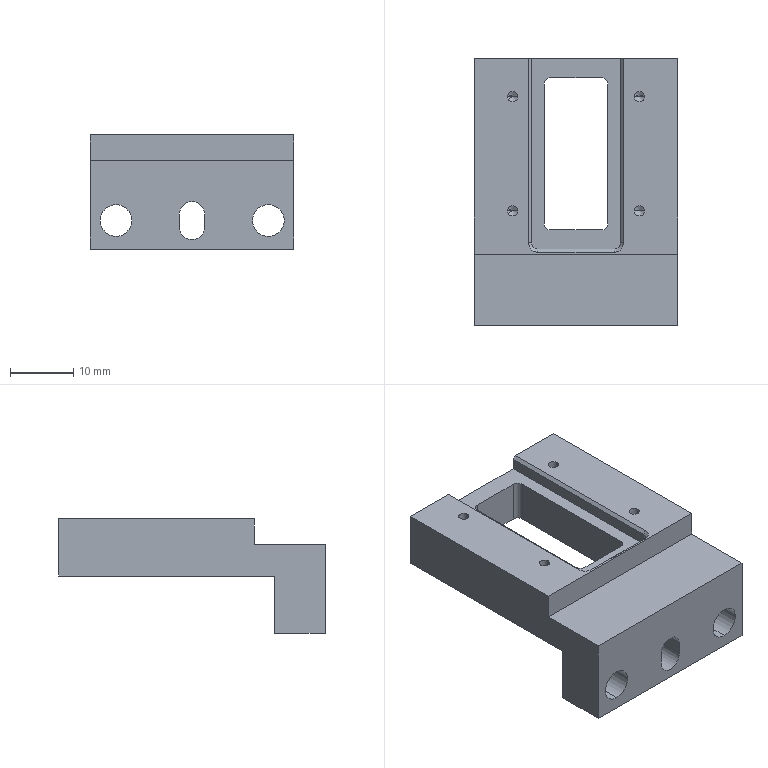NC program | NX | posted with a generic post | part box 32 x 42 x 18 mm
Whole program:
N10 G17 G21 G94 G90
(FLOOR_WALL , TOOL : D10JING)
N12 T11 M6
N14 G54
N16 G17 G0 G90 X-31. Y17.997 B0. C0. S9500 M3
N18 G43 Z30. H11
N20 Z3.
N22 G94 G1 Z0. F1250.
N24 X-28.
N26 X28.
N28 Y13.426
N30 X-28.
N32 Y8.855
N34 X28.
N36 Y4.284
N38 X-28.
N40 Y-0.287
N42 X28.
N44 Y-4.858
N46 X-28.
N48 Y-9.429
N50 X28.
N52 Y-14.
N54 X-28.
N56 X-31.
N58 Z3.
N60 G0 Z30.
N62 M5
(DRILLING , TOOL : D6A45)
N64 T07 M6
N66 G54
N68 G17 G0 G90 X-2.991 Y-10. B0. C0. S5000 M3
N70 G43 Z30. H7
N72 G94 G81 G98 Z-1. F250. R3.
N74 X15.009
N76 Y10.
N78 X-2.991
N80 G80
N82 G0 X-2.991 Y10. Z30.
N84 M5
(DRILLING_COPY , TOOL : 1.6ZT)
N86 T14 M6
N88 G54
N90 G17 G0 G90 X-2.991 Y-10. B0. C0. S2009 M3
N92 G43 Z30. H14
N94 G94 G83 G98 Z-5.681 F100. Q2. R3.
N96 X15.009
N98 Y10.
N100 X-2.991
N102 G80
N104 G0 X-2.991 Y10. Z30.
N106 M5
(ZLEVEL_PROFILE , TOOL : D10)
N108 T10 M6
N110 G54
N112 G17 G0 G90 X-26.1 Y-14.091 B0. C0. S9500 M3
N114 G43 Z30. H10
N116 Z1.5
N118 G94 G1 Y16.32 Z-0.094 F1000.
N120 X-25.983 Y17.131 Z-0.137
N122 X-25.738 Y17.914 Z-0.18
N124 X-25.371 Y18.647 Z-0.223
N126 X-24.892 Y19.312 Z-0.266
N128 X-24.312 Y19.892 Z-0.309
N130 X-23.647 Y20.371 Z-0.352
N132 X-22.914 Y20.738 Z-0.395
N134 X-22.131 Y20.983 Z-0.438
N136 X-21.32 Y21.1 Z-0.48
N138 X-21. Z-0.497
N140 X21. F3000.
N142 G2 X26.1 Y16. R5.1
N144 G1 Y-16.
N146 G2 X21. Y-21.1 R5.1
N148 G1 X-21.
N150 G2 X-26.1 Y-16. R5.1
N152 G1 Y16.
N154 G2 X-21. Y21.1 R5.1
N156 G1 X7.486 Z-0.994
N158 X21.
N160 G2 X26.1 Y16. R5.1
N162 G1 Y-16.
N164 G2 X21. Y-21.1 R5.1
N166 G1 X-21.
N168 G2 X-26.1 Y-16. R5.1
N170 G1 Y16.
N172 G2 X-21. Y21.1 R5.1
N174 G1 X7.486 Z-1.492
N176 X21.
N178 G2 X26.1 Y16. R5.1
N180 G1 Y-16.
N182 G2 X21. Y-21.1 R5.1
N184 G1 X-21.
N186 G2 X-26.1 Y-16. R5.1
N188 G1 Y16.
N190 G2 X-21. Y21.1 R5.1
N192 G1 X7.486 Z-1.989
N194 X21.
N196 G2 X26.1 Y16. R5.1
N198 G1 Y-16.
N200 G2 X21. Y-21.1 R5.1
N202 G1 X-21.
N204 G2 X-26.1 Y-16. R5.1
N206 G1 Y16.
N208 G2 X-21. Y21.1 R5.1
N210 G1 X7.486 Z-2.486
N212 X21.
N214 G2 X26.1 Y16. R5.1
N216 G1 Y-16.
N218 G2 X21. Y-21.1 R5.1
N220 G1 X-21.
N222 G2 X-26.1 Y-16. R5.1
N224 G1 Y16.
N226 G2 X-21. Y21.1 R5.1
N228 G1 X7.486 Z-2.983
N230 X21.
N232 G2 X26.1 Y16. R5.1
N234 G1 Y-16.
N236 G2 X21. Y-21.1 R5.1
N238 G1 X-21.
N240 G2 X-26.1 Y-16. R5.1
N242 G1 Y16.
N244 G2 X-21. Y21.1 R5.1
N246 G1 X7.486 Z-3.481
N248 X21.
N250 G2 X26.1 Y16. R5.1
N252 G1 Y-16.
N254 G2 X21. Y-21.1 R5.1
N256 G1 X-21.
N258 G2 X-26.1 Y-16. R5.1
N260 G1 Y16.
N262 G2 X-21. Y21.1 R5.1
N264 G1 X7.486 Z-3.978
N266 X21.
N268 G2 X26.1 Y16. R5.1
N270 G1 Y-16.
N272 G2 X21. Y-21.1 R5.1
N274 G1 X-21.
N276 G2 X-26.1 Y-16. R5.1
N278 G1 Y16.
N280 G2 X-21. Y21.1 R5.1
N282 G1 X7.486 Z-4.475
N284 X21.
N286 G2 X26.1 Y16. R5.1
N288 G1 Y-16.
N290 G2 X21. Y-21.1 R5.1
N292 G1 X-21.
N294 G2 X-26.1 Y-16. R5.1
N296 G1 Y16.
N298 G2 X-21. Y21.1 R5.1
N300 G1 X7.486 Z-4.972
N302 X21.
N304 G2 X26.1 Y16. R5.1
N306 G1 Y-16.
N308 G2 X21. Y-21.1 R5.1
N310 G1 X-21.
N312 G2 X-26.1 Y-16. R5.1
N314 G1 Y16.
N316 G2 X-21. Y21.1 R5.1
N318 G1 X7.486 Z-5.469
N320 X21.
N322 G2 X26.1 Y16. R5.1
N324 G1 Y-16.
N326 G2 X21. Y-21.1 R5.1
N328 G1 X-21.
N330 G2 X-26.1 Y-16. R5.1
N332 G1 Y16.
N334 G2 X-21. Y21.1 R5.1
N336 G1 X7.486 Z-5.967
N338 X21.
N340 G2 X26.1 Y16. R5.1
N342 G1 Y-16.
N344 G2 X21. Y-21.1 R5.1
N346 G1 X-21.
N348 G2 X-26.1 Y-16. R5.1
N350 G1 Y16.
N352 G2 X-21. Y21.1 R5.1
N354 G1 X7.486 Z-6.464
N356 X21.
N358 G2 X26.1 Y16. R5.1
N360 G1 Y-16.
N362 G2 X21. Y-21.1 R5.1
N364 G1 X-21.
N366 G2 X-26.1 Y-16. R5.1
N368 G1 Y16.
N370 G2 X-21. Y21.1 R5.1
N372 G1 X7.486 Z-6.961
N374 X21.
N376 G2 X26.1 Y16. R5.1
N378 G1 Y-16.
N380 G2 X21. Y-21.1 R5.1
N382 G1 X-21.
N384 G2 X-26.1 Y-16. R5.1
N386 G1 Y16.
N388 G2 X-21. Y21.1 R5.1
N390 G1 X7.486 Z-7.458
N392 X21.
N394 G2 X26.1 Y16. R5.1
N396 G1 Y-16.
N398 G2 X21. Y-21.1 R5.1
N400 G1 X-21.
N402 G2 X-26.1 Y-16. R5.1
N404 G1 Y16.
N406 G2 X-21. Y21.1 R5.1
N408 G1 X7.486 Z-7.956
N410 X21.
N412 G2 X26.1 Y16. R5.1
N414 G1 Y-16.
N416 G2 X21. Y-21.1 R5.1
N418 G1 X-21.
N420 G2 X-26.1 Y-16. R5.1
N422 G1 Y16.
N424 G2 X-21. Y21.1 R5.1
N426 G1 X7.486 Z-8.453
N428 X21.
N430 G2 X26.1 Y16. R5.1
N432 G1 Y-16.
N434 G2 X21. Y-21.1 R5.1
N436 G1 X-21.
N438 G2 X-26.1 Y-16. R5.1
N440 G1 Y16.
N442 G2 X-21. Y21.1 R5.1
N444 G1 X7.486 Z-8.95
N446 X21.
N448 G2 X26.1 Y16. R5.1
N450 G1 Y-16.
N452 G2 X21. Y-21.1 R5.1
N454 G1 X-21.
N456 G2 X-26.1 Y-16. R5.1
N458 G1 Y16.
N460 G2 X-21. Y21.1 R5.1
N462 G1 X7.486 Z-9.447
N464 X21.
N466 G2 X26.1 Y16. R5.1
N468 G1 Y-16.
N470 G2 X21. Y-21.1 R5.1
N472 G1 X-21.
N474 G2 X-26.1 Y-16. R5.1
N476 G1 Y16.
N478 G2 X-21. Y21.1 R5.1
N480 G1 X7.486 Z-9.944
N482 X21.
N484 G2 X26.1 Y16. R5.1
N486 G1 Y-16.
N488 G2 X21. Y-21.1 R5.1
N490 G1 X-21.
N492 G2 X-26.1 Y-16. R5.1
N494 G1 Y16.
N496 G2 X-21. Y21.1 R5.1
N498 G1 X7.486 Z-10.442
N500 X21.
N502 G2 X26.1 Y16. R5.1
N504 G1 Y-16.
N506 G2 X21. Y-21.1 R5.1
N508 G1 X-21.
N510 G2 X-26.1 Y-16. R5.1
N512 G1 Y16.
N514 G2 X-21. Y21.1 R5.1
N516 G1 X7.486 Z-10.939
N518 X21.
N520 G2 X26.1 Y16. R5.1
N522 G1 Y-16.
N524 G2 X21. Y-21.1 R5.1
N526 G1 X-21.
N528 G2 X-26.1 Y-16. R5.1
N530 G1 Y16.
N532 G2 X-21. Y21.1 R5.1
N534 G1 X7.486 Z-11.436
N536 X21.
N538 G2 X26.1 Y16. R5.1
N540 G1 Y-16.
N542 G2 X21. Y-21.1 R5.1
N544 G1 X-21.
N546 G2 X-26.1 Y-16. R5.1
N548 G1 Y16.
N550 G2 X-21. Y21.1 R5.1
N552 G1 X7.486 Z-11.933
N554 X21.
N556 G2 X26.1 Y16. R5.1
N558 G1 Y-16.
N560 G2 X21. Y-21.1 R5.1
N562 G1 X-21.
N564 G2 X-26.1 Y-16. R5.1
N566 G1 Y16.
N568 G2 X-21. Y21.1 R5.1
N570 G1 X7.486 Z-12.431
N572 X21.
N574 G2 X26.1 Y16. R5.1
N576 G1 Y-16.
N578 G2 X21. Y-21.1 R5.1
N580 G1 X-21.
N582 G2 X-26.1 Y-16. R5.1
N584 G1 Y16.
N586 G2 X-21. Y21.1 R5.1
N588 G1 X7.486 Z-12.928
N590 X21.
N592 G2 X26.1 Y16. R5.1
N594 G1 Y-16.
N596 G2 X21. Y-21.1 R5.1
N598 G1 X-21.
N600 G2 X-26.1 Y-16. R5.1
N602 G1 Y16.
N604 G2 X-21. Y21.1 R5.1
N606 G1 X7.486 Z-13.425
N608 X21.
N610 G2 X26.1 Y16. R5.1
N612 G1 Y-16.
N614 G2 X21. Y-21.1 R5.1
N616 G1 X-21.
N618 G2 X-26.1 Y-16. R5.1
N620 G1 Y16.
N622 G2 X-21. Y21.1 R5.1
N624 G1 X7.486 Z-13.922
N626 X21.
N628 G2 X26.1 Y16. R5.1
N630 G1 Y-16.
N632 G2 X21. Y-21.1 R5.1
N634 G1 X-21.
N636 G2 X-26.1 Y-16. R5.1
N638 G1 Y16.
N640 G2 X-21. Y21.1 R5.1
N642 G1 X7.486 Z-14.419
N644 X21.
N646 G2 X26.1 Y16. R5.1
N648 G1 Y-16.
N650 G2 X21. Y-21.1 R5.1
N652 G1 X-21.
N654 G2 X-26.1 Y-16. R5.1
N656 G1 Y16.
N658 G2 X-21. Y21.1 R5.1
N660 G1 X7.486 Z-14.917
N662 X21.
N664 G2 X26.1 Y16. R5.1
N666 G1 Y-16.
N668 G2 X21. Y-21.1 R5.1
N670 G1 X-21.
N672 G2 X-26.1 Y-16. R5.1
N674 G1 Y16.
N676 G2 X-21. Y21.1 R5.1
N678 G1 X7.486 Z-15.414
N680 X21.
N682 G2 X26.1 Y16. R5.1
N684 G1 Y-16.
N686 G2 X21. Y-21.1 R5.1
N688 G1 X-21.
N690 G2 X-26.1 Y-16. R5.1
N692 G1 Y16.
N694 G2 X-21. Y21.1 R5.1
N696 G1 X7.486 Z-15.911
N698 X21.
N700 G2 X26.1 Y16. R5.1
N702 G1 Y-16.
N704 G2 X21. Y-21.1 R5.1
N706 G1 X-21.
N708 G2 X-26.1 Y-16. R5.1
N710 G1 Y16.
N712 G2 X-21. Y21.1 R5.1
N714 G1 X7.486 Z-16.408
N716 X21.
N718 G2 X26.1 Y16. R5.1
N720 G1 Y-16.
N722 G2 X21. Y-21.1 R5.1
N724 G1 X-21.
N726 G2 X-26.1 Y-16. R5.1
N728 G1 Y16.
N730 G2 X-21. Y21.1 R5.1
N732 G1 X7.486 Z-16.906
N734 X21.
N736 G2 X26.1 Y16. R5.1
N738 G1 Y-16.
N740 G2 X21. Y-21.1 R5.1
N742 G1 X-21.
N744 G2 X-26.1 Y-16. R5.1
N746 G1 Y16.
N748 G2 X-21. Y21.1 R5.1
N750 G1 X7.486 Z-17.403
N752 X21.
N754 G2 X26.1 Y16. R5.1
N756 G1 Y-16.
N758 G2 X21. Y-21.1 R5.1
N760 G1 X-21.
N762 G2 X-26.1 Y-16. R5.1
N764 G1 Y16.
N766 G2 X-21. Y21.1 R5.1
N768 G1 X7.486 Z-17.9
N770 X21.
N772 G2 X26.1 Y16. R5.1
N774 G1 Y-16.
N776 G2 X21. Y-21.1 R5.1
N778 G1 X-21.
N780 G2 X-26.1 Y-16. R5.1
N782 G1 Y16.
N784 G2 X-21. Y21.1 R5.1
N786 G1 X7.486
N788 Z-16.4
N790 G0 Z30.
N792 M5
(ZLEVEL_PROFILE_COPY_1 , TOOL : D10JING)
N794 T11 M6
N796 G54
N798 G17 G0 G90 X-22.622 Y22.809 B0. C0. S9500 M3
N800 G43 Z30. H11
N802 Z-16.4
N804 G94 G1 Z-17.9 F1000.
N806 X-21.866 Y21.5
N808 G3 X-21. Y21. R1.
N810 G1 X21. F1200.
N812 G2 X26. Y16. R5.
N814 G1 Y-16.
N816 G2 X21. Y-21. R5.
N818 G1 X-21.
N820 G2 X-26. Y-16. R5.
N822 G1 Y16.
N824 G2 X-21. Y21. R5.
N826 G3 X-20.134 Y21.5 R1.
N828 G1 X-19.268 Y23.
N830 Z-16.4
N832 G0 Z30.
N834 M5
(FLOOR_WALL_1 , TOOL : D6)
N836 T06 M6
N838 G54
N840 G17 G0 G90 X-25. Y-3.636 B0. C0. S9500 M3
N842 G43 Z30. H6
N844 Z0.513
N846 G94 G1 Z-0.488 F1000.
N848 X-21.214 Y-0.46
N850 G3 X-21. Y0. R0.6
N852 G1 Y16. F2500.
N854 X-12.9
N856 Y-16.
N858 X-21.
N860 Y0.
N862 X-18.3
N864 Y13.3
N866 X-15.6
N868 Y-13.3
N870 X-18.3
N872 Y0.
N874 G3 X-18.514 Y0.46 R0.6
N876 G1 Z0.513
N878 G0 X-25. Y-3.636 Z0.025
N880 G1 Z-0.975 F1000.
N882 X-21.214 Y-0.46
N884 G3 X-21. Y0. R0.6
N886 G1 Y16. F2500.
N888 X-12.9
N890 Y-16.
N892 X-21.
N894 Y0.
N896 X-18.3
N898 Y13.3
N900 X-15.6
N902 Y-13.3
N904 X-18.3
N906 Y0.
N908 G3 X-18.514 Y0.46 R0.6
N910 G1 Z0.025
N912 G0 X-25. Y-3.636 Z-0.463
N914 G1 Z-1.463 F1000.
N916 X-21.214 Y-0.46
N918 G3 X-21. Y0. R0.6
N920 G1 Y16. F2500.
N922 X-12.9
N924 Y-16.
N926 X-21.
N928 Y0.
N930 X-18.3
N932 Y13.3
N934 X-15.6
N936 Y-13.3
N938 X-18.3
N940 Y0.
N942 G3 X-18.514 Y0.46 R0.6
N944 G1 Z-0.463
N946 G0 X-25. Y-3.636 Z-0.95
N948 G1 Z-1.95 F1000.
N950 X-21.214 Y-0.46
N952 G3 X-21. Y0. R0.6
N954 G1 Y16. F2500.
N956 X-12.9
N958 Y-16.
N960 X-21.
N962 Y0.
N964 X-18.3
N966 Y13.3
N968 X-15.6
N970 Y-13.3
N972 X-18.3
N974 Y0.
N976 G3 X-18.514 Y0.46 R0.6
N978 G1 Z-0.95
N980 G0 X-25. Y-3.636 Z-1.438
N982 G1 Z-2.438 F1000.
N984 X-21.214 Y-0.46
N986 G3 X-21. Y0. R0.6
N988 G1 Y16. F2500.
N990 X-12.9
N992 Y-16.
N994 X-21.
N996 Y0.
N998 X-18.3
N1000 Y13.3
N1002 X-15.6
N1004 Y-13.3
N1006 X-18.3
N1008 Y0.
N1010 G3 X-18.514 Y0.46 R0.6
N1012 G1 Z-1.438
N1014 G0 X-25. Y-3.636 Z-1.925
N1016 G1 Z-2.925 F1000.
N1018 X-21.214 Y-0.46
N1020 G3 X-21. Y0. R0.6
N1022 G1 Y16. F2500.
N1024 X-12.9
N1026 Y-16.
N1028 X-21.
N1030 Y0.
N1032 X-18.3
N1034 Y13.3
N1036 X-15.6
N1038 Y-13.3
N1040 X-18.3
N1042 Y0.
N1044 G3 X-18.514 Y0.46 R0.6
N1046 G1 Z-1.925
N1048 G0 X-25. Y-3.636 Z-2.413
N1050 G1 Z-3.413 F1000.
N1052 X-21.214 Y-0.46
N1054 G3 X-21. Y0. R0.6
N1056 G1 Y16. F2500.
N1058 X-12.9
N1060 Y-16.
N1062 X-21.
N1064 Y0.
N1066 X-18.3
N1068 Y13.3
N1070 X-15.6
N1072 Y-13.3
N1074 X-18.3
N1076 Y0.
N1078 G3 X-18.514 Y0.46 R0.6
N1080 G1 Z-2.413
N1082 G0 X-25. Y-3.636 Z-2.9
N1084 G1 Z-3.9 F1000.
N1086 X-21.214 Y-0.46
N1088 G3 X-21. Y0. R0.6
N1090 G1 Y16. F2500.
N1092 X-12.9
N1094 Y-16.
N1096 X-21.
N1098 Y0.
N1100 X-18.3
N1102 Y13.3
N1104 X-15.6
N1106 Y-13.3
N1108 X-18.3
N1110 Y0.
N1112 G3 X-18.514 Y0.46 R0.6
N1114 G1 Z-2.9
N1116 G0 Z30.
(FLOOR_WALL_1_COPY , TOOL : D6)
N1118 X25.
N1120 Z0.56
N1122 G1 Z-0.44 F1000.
N1124 X21.214
N1126 G3 X21. Y0. R0.6
N1128 G1 Y-3.9 F2500.
N1130 X-5.9
N1132 Y3.9
N1134 X21.
N1136 Y0.
N1138 X18.3
N1140 Y-1.2
N1142 X-3.2
N1144 Y1.2
N1146 X18.3
N1148 Y0.
N1150 G3 X18.514 Y-0.46 R0.6
N1152 G1 Z0.56
N1154 G0 X25. Y0.46 Z0.12
N1156 G1 Z-0.88 F1000.
N1158 X21.214
N1160 G3 X21. Y0. R0.6
N1162 G1 Y-3.9 F2500.
N1164 X-5.9
N1166 Y3.9
N1168 X21.
N1170 Y0.
N1172 X18.3
N1174 Y-1.2
N1176 X-3.2
N1178 Y1.2
N1180 X18.3
N1182 Y0.
N1184 G3 X18.514 Y-0.46 R0.6
N1186 G1 Z0.12
N1188 G0 X25. Y0.46 Z-0.32
N1190 G1 Z-1.32 F1000.
N1192 X21.214
N1194 G3 X21. Y0. R0.6
N1196 G1 Y-3.9 F2500.
N1198 X-5.9
N1200 Y3.9
N1202 X21.
N1204 Y0.
N1206 X18.3
N1208 Y-1.2
N1210 X-3.2
N1212 Y1.2
N1214 X18.3
N1216 Y0.
N1218 G3 X18.514 Y-0.46 R0.6
N1220 G1 Z-0.32
N1222 G0 X25. Y0.46 Z-0.76
N1224 G1 Z-1.76 F1000.
N1226 X21.214
N1228 G3 X21. Y0. R0.6
N1230 G1 Y-3.9 F2500.
N1232 X-5.9
N1234 Y3.9
N1236 X21.
N1238 Y0.
N1240 X18.3
N1242 Y-1.2
N1244 X-3.2
N1246 Y1.2
N1248 X18.3
N1250 Y0.
N1252 G3 X18.514 Y-0.46 R0.6
N1254 G1 Z-0.76
N1256 G0 X25. Y0.46 Z-1.2
N1258 G1 Z-2.2 F1000.
N1260 X21.214
N1262 G3 X21. Y0. R0.6
N1264 G1 Y-3.9 F2500.
N1266 X-5.9
N1268 Y3.9
N1270 X21.
N1272 Y0.
N1274 X18.3
N1276 Y-1.2
N1278 X-3.2
N1280 Y1.2
N1282 X18.3
N1284 Y0.
N1286 G3 X18.514 Y-0.46 R0.6
N1288 G1 Z-1.2
N1290 G0 Z30.
(ZLEVEL_PROFILE_COPY , TOOL : D6)
N1292 X9.451 Y1.9
N1294 Z-0.8
N1296 G1 X-2.9 Z-1.447 F1000.
N1298 Y-1.9 Z-1.646
N1300 X14.902 Z-2.579
N1302 X14.9 Y-1.851 Z-2.582
N1304 Y1.9 Z-2.779
N1306 X-2.9 F2200.
N1308 Y-1.9
N1310 X14.902
N1312 X14.9 Y-1.851
N1314 Y1.9
N1316 X-2.861 Z-3.089
N1318 X-2.9 Y1.767 Z-3.092
N1320 Y-1.855 Z-3.155
N1322 X-2.773 Y-1.9 Z-3.158
N1324 X2.917 Z-3.257
N1326 X14.902
N1328 X14.9 Y-1.851
N1330 Y1.9
N1332 X-2.861 Z-3.567
N1334 X-2.9 Y1.767 Z-3.57
N1336 Y-1.855 Z-3.633
N1338 X-2.773 Y-1.9 Z-3.636
N1340 X2.917 Z-3.736
N1342 X14.902
N1344 X14.9 Y-1.851
N1346 Y1.9
N1348 X-2.861 Z-4.046
N1350 X-2.9 Y1.767 Z-4.049
N1352 Y-1.855 Z-4.112
N1354 X-2.773 Y-1.9 Z-4.115
N1356 X2.917 Z-4.214
N1358 X14.902
N1360 X14.9 Y-1.851
N1362 Y1.9
N1364 X-2.861 Z-4.524
N1366 X-2.9 Y1.767 Z-4.527
N1368 Y-1.855 Z-4.591
N1370 X-2.773 Y-1.9 Z-4.594
N1372 X2.917 Z-4.693
N1374 X14.902
N1376 X14.9 Y-1.851
N1378 Y1.9
N1380 X-2.861 Z-5.003
N1382 X-2.9 Y1.767 Z-5.006
N1384 Y-1.855 Z-5.069
N1386 X-2.773 Y-1.9 Z-5.072
N1388 X2.917 Z-5.171
N1390 X14.902
N1392 X14.9 Y-1.851
N1394 Y1.9
N1396 X-2.861 Z-5.481
N1398 X-2.9 Y1.767 Z-5.484
N1400 Y-1.855 Z-5.548
N1402 X-2.773 Y-1.9 Z-5.551
N1404 X2.917 Z-5.65
N1406 X14.902
N1408 X14.9 Y-1.851
N1410 Y1.9
N1412 X-2.861 Z-5.96
N1414 X-2.9 Y1.767 Z-5.963
N1416 Y-1.855 Z-6.026
N1418 X-2.773 Y-1.9 Z-6.029
N1420 X2.917 Z-6.129
N1422 X14.902
N1424 X14.9 Y-1.851
N1426 Y1.9
N1428 X-2.861 Z-6.439
N1430 X-2.9 Y1.767 Z-6.442
N1432 Y-1.855 Z-6.505
N1434 X-2.773 Y-1.9 Z-6.508
N1436 X2.917 Z-6.607
N1438 X14.902
N1440 X14.9 Y-1.851
N1442 Y1.9
N1444 X-2.861 Z-6.917
N1446 X-2.9 Y1.767 Z-6.92
N1448 Y-1.855 Z-6.983
N1450 X-2.773 Y-1.9 Z-6.986
N1452 X2.917 Z-7.086
N1454 X14.902
N1456 X14.9 Y-1.851
N1458 Y1.9
N1460 X-2.861 Z-7.396
N1462 X-2.9 Y1.767 Z-7.399
N1464 Y-1.855 Z-7.462
N1466 X-2.773 Y-1.9 Z-7.465
N1468 X2.917 Z-7.564
N1470 X14.902
N1472 X14.9 Y-1.851
N1474 Y1.9
N1476 X-2.861 Z-7.874
N1478 X-2.9 Y1.767 Z-7.877
N1480 Y-1.855 Z-7.941
N1482 X-2.773 Y-1.9 Z-7.944
N1484 X2.917 Z-8.043
N1486 X14.902
N1488 X14.9 Y-1.851
N1490 Y1.9
N1492 X-2.861 Z-8.353
N1494 X-2.9 Y1.767 Z-8.356
N1496 Y-1.855 Z-8.419
N1498 X-2.773 Y-1.9 Z-8.422
N1500 X2.917 Z-8.521
N1502 X14.902
N1504 X14.9 Y-1.851
N1506 Y1.9
N1508 X-2.861 Z-8.831
N1510 X-2.9 Y1.767 Z-8.834
N1512 Y-1.855 Z-8.898
N1514 X-2.773 Y-1.9 Z-8.901
N1516 X2.917 Z-9.
N1518 X14.902
N1520 X14.9 Y-1.851
N1522 Y1.9
N1524 X-2.9
N1526 Y-1.9
N1528 X2.917
N1530 Z-7.5
N1532 G0 Z30.
(FLOOR_WALL_1_1_COPY , TOOL : D6)
N1534 X25.5 Y-3.399
N1536 Z-0.8
N1538 G1 Z-2.3 F1250.
N1540 X23.48
N1542 G3 X24. Y-3.699 R0.6
N1544 G1 X-5.7
N1546 Y-1.233
N1548 X24.
N1550 Y1.234
N1552 X-5.7
N1554 Y3.7
N1556 X24.
N1558 G2 X24.52 Y3.4 R0.6
N1560 G1 X25.5 Y1.702
N1562 Z-0.8
N1564 G0 Z7.8
N1566 Y2.002
N1568 Z-0.8
N1570 G1 Z-2.3
N1572 X24.52 Y3.7
N1574 G3 X24. Y4. R0.6
N1576 G1 X-6.
N1578 Y-4.
N1580 X24.
N1582 G3 X24.52 Y-3.7 R0.6
N1584 G1 X25.5 Y-2.002
N1586 Z-0.8
N1588 G0 Z30.
(ZLEVEL_PROFILE_COPY_1_COPY , TOOL : D6)
N1590 X13.522 Y0.8
N1592 Z-7.5
N1594 G1 Z-9. F1000.
N1596 X14.7 Y1.48
N1598 G3 X15. Y2. R0.6
N1600 G1 X-3. F1200.
N1602 Y-2.
N1604 X15.
N1606 Y2.
N1608 G3 X14.48 Y1.7 R0.6
N1610 G1 X13.8 Y0.522
N1612 Z-7.5
N1614 G0 Z30.
N1616 M5
(ZLEVEL_PROFILE_COPY_COPY , TOOL : D2)
N1618 T02 M6
N1620 G54
N1622 G17 G0 G90 X-5.793 Y5.956 B0. C0. S9500 M3
N1624 G43 Z30. H2
N1626 Z-0.144
N1628 G94 G1 X-5.967 Y6.256 F1000.
N1630 G3 X-6.14 Y6.356 R0.2
N1632 G1 X-8.
N1634 G3 X-8.356 Y6. R0.356
N1636 G1 Y4.14
N1638 G3 X-8.256 Y3.967 R0.2
N1640 G1 X-7.956 Y3.793
N1642 G0 X-5.65 Y5.813 Z-0.288
N1644 G1 X-5.823 Y6.113
N1646 G3 X-5.996 Y6.213 R0.2
N1648 G1 X-8.
N1650 G3 X-8.213 Y6. R0.213
N1652 G1 Y3.996
N1654 G3 X-8.113 Y3.823 R0.2
N1656 G1 X-7.813 Y3.65
N1658 G0 X-5.506 Y5.669 Z-0.431
N1660 G1 X-5.679 Y5.969
N1662 G3 X-5.852 Y6.069 R0.2
N1664 G1 X-8.
N1666 X-8.039 Y6.068
N1668 X-8.068 Y6.039
N1670 X-8.069 Y6.
N1672 Y3.852
N1674 G3 X-7.969 Y3.679 R0.2
N1676 G1 X-7.669 Y3.506
N1678 G0 X-5.437 Y5.6 Z-0.575
N1680 G1 X-5.61 Y5.9
N1682 G3 X-5.784 Y6. R0.2
N1684 G1 X-8.
N1686 Y3.784
N1688 G3 X-7.9 Y3.61 R0.2
N1690 G1 X-7.6 Y3.437
N1692 G0 X-5.437 Y5.6 Z-0.719
N1694 G1 X-5.61 Y5.9
N1696 G3 X-5.784 Y6. R0.2
N1698 G1 X-8.
N1700 Y3.784
N1702 G3 X-7.9 Y3.61 R0.2
N1704 G1 X-7.6 Y3.437
N1706 G0 X-5.437 Y5.6 Z-0.863
N1708 G1 X-5.61 Y5.9
N1710 G3 X-5.784 Y6. R0.2
N1712 G1 X-8.
N1714 Y3.784
N1716 G3 X-7.9 Y3.61 R0.2
N1718 G1 X-7.6 Y3.437
N1720 G0 X-5.437 Y5.6 Z-1.006
N1722 G1 X-5.61 Y5.9
N1724 G3 X-5.784 Y6. R0.2
N1726 G1 X-8.
N1728 Y3.784
N1730 G3 X-7.9 Y3.61 R0.2
N1732 G1 X-7.6 Y3.437
N1734 G0 X-5.437 Y5.6 Z-1.15
N1736 G1 X-5.61 Y5.9
N1738 G3 X-5.784 Y6. R0.2
N1740 G1 X-8.
N1742 Y3.784
N1744 G3 X-7.9 Y3.61 R0.2
N1746 G1 X-7.6 Y3.437
N1748 G0 X-5.437 Y5.6 Z-1.294
N1750 G1 X-5.61 Y5.9
N1752 G3 X-5.784 Y6. R0.2
N1754 G1 X-8.
N1756 Y3.784
N1758 G3 X-7.9 Y3.61 R0.2
N1760 G1 X-7.6 Y3.437
N1762 G0 X-5.437 Y5.6 Z-1.438
N1764 G1 X-5.61 Y5.9
N1766 G3 X-5.784 Y6. R0.2
N1768 G1 X-8.
N1770 Y3.784
N1772 G3 X-7.9 Y3.61 R0.2
N1774 G1 X-7.6 Y3.437
N1776 G0 X-5.437 Y5.6 Z-1.581
N1778 G1 X-5.61 Y5.9
N1780 G3 X-5.784 Y6. R0.2
N1782 G1 X-8.
N1784 Y3.784
N1786 G3 X-7.9 Y3.61 R0.2
N1788 G1 X-7.6 Y3.437
N1790 G0 X-5.437 Y5.6 Z-1.725
N1792 G1 X-5.61 Y5.9
N1794 G3 X-5.784 Y6. R0.2
N1796 G1 X-8.
N1798 Y3.784
N1800 G3 X-7.9 Y3.61 R0.2
N1802 G1 X-7.6 Y3.437
N1804 G0 X-5.437 Y5.6 Z-1.869
N1806 G1 X-5.61 Y5.9
N1808 G3 X-5.784 Y6. R0.2
N1810 G1 X-8.
N1812 Y3.784
N1814 G3 X-7.9 Y3.61 R0.2
N1816 G1 X-7.6 Y3.437
N1818 G0 X-5.437 Y5.6 Z-2.013
N1820 G1 X-5.61 Y5.9
N1822 G3 X-5.784 Y6. R0.2
N1824 G1 X-8.
N1826 Y3.784
N1828 G3 X-7.9 Y3.61 R0.2
N1830 G1 X-7.6 Y3.437
N1832 G0 X-5.437 Y5.6 Z-2.156
N1834 G1 X-5.61 Y5.9
N1836 G3 X-5.784 Y6. R0.2
N1838 G1 X-8.
N1840 Y3.784
N1842 G3 X-7.9 Y3.61 R0.2
N1844 G1 X-7.6 Y3.437
N1846 G0 X-5.437 Y5.6 Z-2.3
N1848 G1 X-5.61 Y5.9
N1850 G3 X-5.784 Y6. R0.2
N1852 G1 X-8.
N1854 Y3.784
N1856 G3 X-7.9 Y3.61 R0.2
N1858 G1 X-7.6 Y3.437
N1860 G0 Z30.
N1862 X-7.956 Y-3.793
N1864 Z-0.144
N1866 G1 X-8.256 Y-3.967
N1868 G3 X-8.356 Y-4.14 R0.2
N1870 G1 Y-6.
N1872 G3 X-8. Y-6.356 R0.356
N1874 G1 X-6.14
N1876 G3 X-5.967 Y-6.256 R0.2
N1878 G1 X-5.793 Y-5.956
N1880 G0 X-7.813 Y-3.65 Z-0.288
N1882 G1 X-8.113 Y-3.823
N1884 G3 X-8.213 Y-3.996 R0.2
N1886 G1 Y-6.
N1888 G3 X-8. Y-6.213 R0.213
N1890 G1 X-5.996
N1892 G3 X-5.823 Y-6.113 R0.2
N1894 G1 X-5.65 Y-5.813
N1896 G0 X-7.669 Y-3.506 Z-0.431
N1898 G1 X-7.969 Y-3.679
N1900 G3 X-8.069 Y-3.852 R0.2
N1902 G1 Y-6.
N1904 X-8.068 Y-6.039
N1906 X-8.039 Y-6.068
N1908 X-8. Y-6.069
N1910 X-5.852
N1912 G3 X-5.679 Y-5.969 R0.2
N1914 G1 X-5.506 Y-5.669
N1916 G0 X-7.6 Y-3.437 Z-0.575
N1918 G1 X-7.9 Y-3.61
N1920 G3 X-8. Y-3.784 R0.2
N1922 G1 Y-6.
N1924 X-5.784
N1926 G3 X-5.61 Y-5.9 R0.2
N1928 G1 X-5.437 Y-5.6
N1930 G0 X-7.6 Y-3.437 Z-0.719
N1932 G1 X-7.9 Y-3.61
N1934 G3 X-8. Y-3.784 R0.2
N1936 G1 Y-6.
N1938 X-5.784
N1940 G3 X-5.61 Y-5.9 R0.2
N1942 G1 X-5.437 Y-5.6
N1944 G0 X-7.6 Y-3.437 Z-0.863
N1946 G1 X-7.9 Y-3.61
N1948 G3 X-8. Y-3.784 R0.2
N1950 G1 Y-6.
N1952 X-5.784
N1954 G3 X-5.61 Y-5.9 R0.2
N1956 G1 X-5.437 Y-5.6
N1958 G0 X-7.6 Y-3.437 Z-1.006
N1960 G1 X-7.9 Y-3.61
N1962 G3 X-8. Y-3.784 R0.2
N1964 G1 Y-6.
N1966 X-5.784
N1968 G3 X-5.61 Y-5.9 R0.2
N1970 G1 X-5.437 Y-5.6
N1972 G0 X-7.6 Y-3.437 Z-1.15
N1974 G1 X-7.9 Y-3.61
N1976 G3 X-8. Y-3.784 R0.2
N1978 G1 Y-6.
N1980 X-5.784
N1982 G3 X-5.61 Y-5.9 R0.2
N1984 G1 X-5.437 Y-5.6
N1986 G0 X-7.6 Y-3.437 Z-1.294
N1988 G1 X-7.9 Y-3.61
N1990 G3 X-8. Y-3.784 R0.2
N1992 G1 Y-6.
N1994 X-5.784
N1996 G3 X-5.61 Y-5.9 R0.2
N1998 G1 X-5.437 Y-5.6
N2000 G0 X-7.6 Y-3.437 Z-1.438
N2002 G1 X-7.9 Y-3.61
N2004 G3 X-8. Y-3.784 R0.2
N2006 G1 Y-6.
N2008 X-5.784
N2010 G3 X-5.61 Y-5.9 R0.2
N2012 G1 X-5.437 Y-5.6
N2014 G0 X-7.6 Y-3.437 Z-1.581
N2016 G1 X-7.9 Y-3.61
N2018 G3 X-8. Y-3.784 R0.2
N2020 G1 Y-6.
N2022 X-5.784
N2024 G3 X-5.61 Y-5.9 R0.2
N2026 G1 X-5.437 Y-5.6
N2028 G0 X-7.6 Y-3.437 Z-1.725
N2030 G1 X-7.9 Y-3.61
N2032 G3 X-8. Y-3.784 R0.2
N2034 G1 Y-6.
N2036 X-5.784
N2038 G3 X-5.61 Y-5.9 R0.2
N2040 G1 X-5.437 Y-5.6
N2042 G0 X-7.6 Y-3.437 Z-1.869
N2044 G1 X-7.9 Y-3.61
N2046 G3 X-8. Y-3.784 R0.2
N2048 G1 Y-6.
N2050 X-5.784
N2052 G3 X-5.61 Y-5.9 R0.2
N2054 G1 X-5.437 Y-5.6
N2056 G0 X-7.6 Y-3.437 Z-2.013
N2058 G1 X-7.9 Y-3.61
N2060 G3 X-8. Y-3.784 R0.2
N2062 G1 Y-6.
N2064 X-5.784
N2066 G3 X-5.61 Y-5.9 R0.2
N2068 G1 X-5.437 Y-5.6
N2070 G0 X-7.6 Y-3.437 Z-2.156
N2072 G1 X-7.9 Y-3.61
N2074 G3 X-8. Y-3.784 R0.2
N2076 G1 Y-6.
N2078 X-5.784
N2080 G3 X-5.61 Y-5.9 R0.2
N2082 G1 X-5.437 Y-5.6
N2084 G0 X-7.6 Y-3.437 Z-2.3
N2086 G1 X-7.9 Y-3.61
N2088 G3 X-8. Y-3.784 R0.2
N2090 G1 Y-6.
N2092 X-5.784
N2094 G3 X-5.61 Y-5.9 R0.2
N2096 G1 X-5.437 Y-5.6
N2098 G0 Z30.
(PLANAR_MILL_COPY_COPY_1 , TOOL : D6A45)
N2100 T07 M6
N2102 G17 G43 G0 G90 X22.27 Y4.8 Z30. B0. C0. S9500 H7 M3
N2104 Z0.
N2106 G94 G1 Z-1.5 F1250.
N2108 X21.866 Y5.5
N2110 G3 X21. Y6. R1.
N2112 G1 X-8.
N2114 Y-6.
N2116 X21.
N2118 G3 X21.866 Y-5.5 R1.
N2120 G1 X22.27 Y-4.8
N2122 Z0.
N2124 G0 Z30.
N2126 M5
(刀补6 , TOOL : D6)
N2128 T06 M6
N2130 G54
N2132 G17 G0 G90 X25.247 Y2.406 B0. C0. S9500 M3
N2134 G43 Z30. H6
N2136 Z-0.8
N2138 G94 G1 Z-2.3 F1250.
N2140 G41 X25.212 Y2.5 D6
N2142 X24.52 Y3.7
N2144 G3 X24. Y4. R0.6
N2146 G1 X-6.
N2148 Y-4.
N2150 X24.
N2152 G3 X24.52 Y-3.7 R0.6
N2154 G1 X25.212 Y-2.5
N2156 G40
N2158 X25.247 Y-2.406
N2160 Z-0.8
N2162 G0 Z30.
N2164 M5
N2166 M2